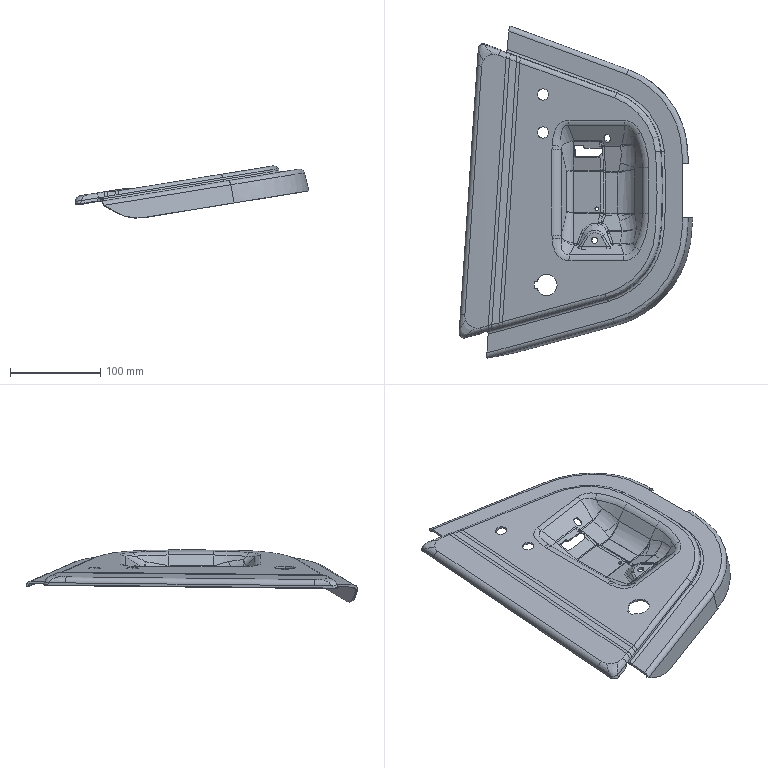Part | SolidWorks | features BaseBody 1 | 1 solid | 397 faces | box 258.18 x 367.01 x 57.896 mm | volume 192085 mm3 | spline 164 | cylinder 117 | plane 72 | torus 23 | sphere 12 | cone 9 | commonest cylinder face diameters 14.6 x15 10 x14 10.6 x13 6 x12 9.2 x9 4.6 x8